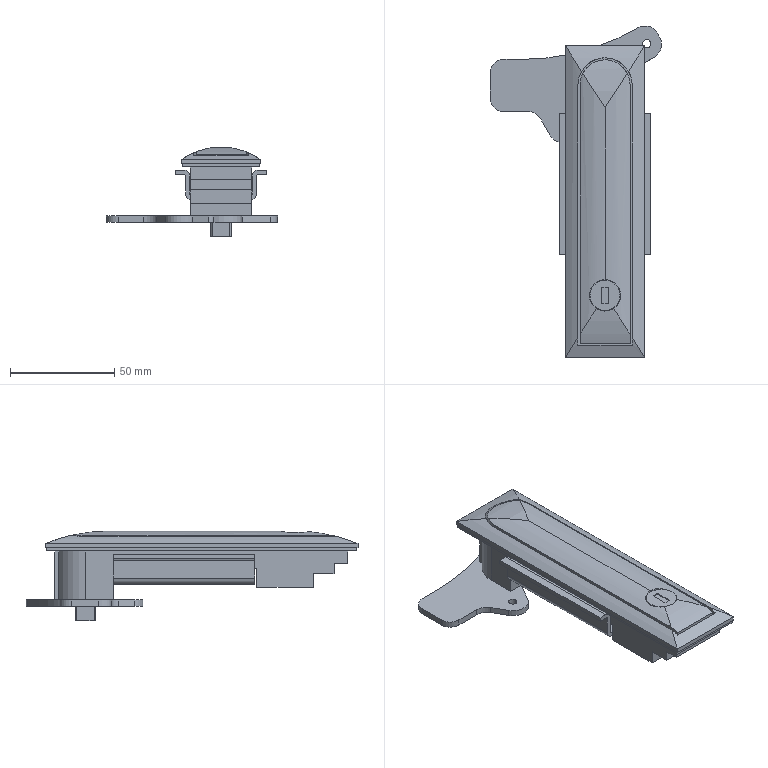Part | NX | features BREP 3 | 3 solids | 144 faces | box 82.16 x 159.283 x 43 mm | volume 107994 mm3 | plane 73 | cylinder 65 | cone 6 | commonest cylinder face diameters 4 x10 4.2 x10 2 x9 6 x4 13 x4 14 x4